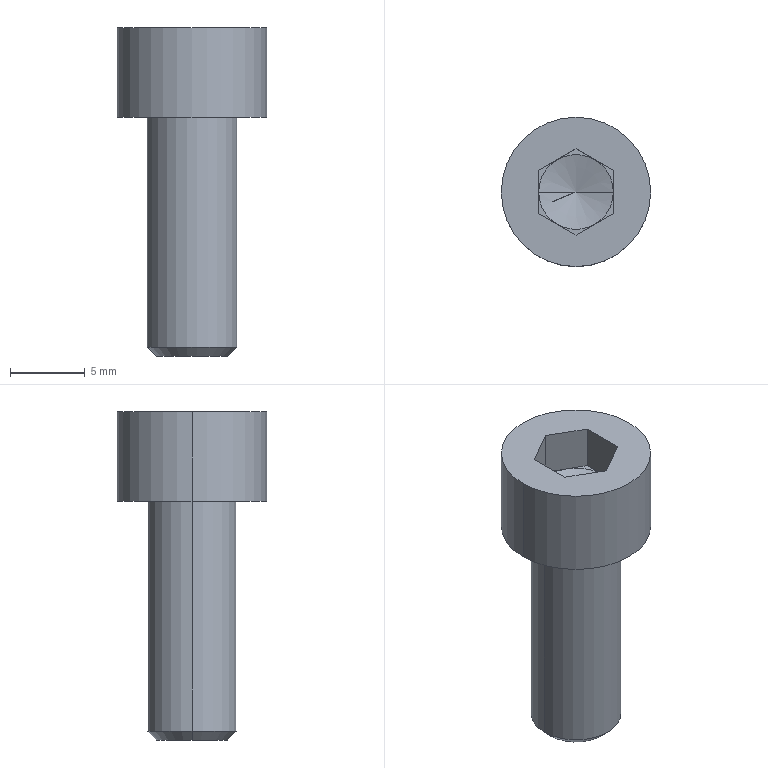Part | STEP file | TNSN20-Y20-F22-Part-7 | 1 solid | 23 faces | box 10 x 10 x 22 mm | volume 850.987 mm3 | plane 15 | cylinder 4 | cone 4 | commonest cylinder face diameters 6 x2 10 x2
STEP:
#1=CARTESIAN_POINT('',(14087.745,13740.046,22.6));
#2=VERTEX_POINT('',#1);
#3=CARTESIAN_POINT('',(14097.745,13740.046,22.6));
#4=VERTEX_POINT('',#3);
#5=CARTESIAN_POINT('',(14092.745,13740.046,22.6));
#6=DIRECTION('',(0.,0.,-1.));
#7=DIRECTION('',(1.,0.,0.));
#8=AXIS2_PLACEMENT_3D('',#5,#6,#7);
#9=CIRCLE('',#8,5.);
#10=EDGE_CURVE('',#2,#4,#9,.T.);
#11=ORIENTED_EDGE('',*,*,#10,.F.);
#12=CARTESIAN_POINT('',(14092.745,13740.046,22.6));
#13=DIRECTION('',(0.,0.,-1.));
#14=DIRECTION('',(1.,0.,0.));
#15=AXIS2_PLACEMENT_3D('',#12,#13,#14);
#16=CIRCLE('',#15,5.);
#17=EDGE_CURVE('',#4,#2,#16,.T.);
#18=ORIENTED_EDGE('',*,*,#17,.F.);
#19=EDGE_LOOP('',(#11,#18));
#20=FACE_OUTER_BOUND('',#19,.T.);
#21=CARTESIAN_POINT('',(14092.745,13742.933,22.6));
#22=VERTEX_POINT('',#21);
#23=CARTESIAN_POINT('',(14095.245,13741.49,22.6));
#24=VERTEX_POINT('',#23);
#25=CARTESIAN_POINT('',(14092.745,13742.933,22.6));
#26=DIRECTION('',(0.866,-0.5,0.));
#27=VECTOR('',#26,1000.);
#28=LINE('',#25,#27);
#29=EDGE_CURVE('',#22,#24,#28,.T.);
#30=ORIENTED_EDGE('',*,*,#29,.T.);
#31=CARTESIAN_POINT('',(14095.245,13738.603,22.6));
#32=VERTEX_POINT('',#31);
#33=CARTESIAN_POINT('',(14095.245,13741.49,22.6));
#34=DIRECTION('',(0.,-1.,0.));
#35=VECTOR('',#34,1000.);
#36=LINE('',#33,#35);
#37=EDGE_CURVE('',#24,#32,#36,.T.);
#38=ORIENTED_EDGE('',*,*,#37,.T.);
#39=CARTESIAN_POINT('',(14092.745,13737.16,22.6));
#40=VERTEX_POINT('',#39);
#41=CARTESIAN_POINT('',(14095.245,13738.603,22.6));
#42=DIRECTION('',(-0.866,-0.5,0.));
#43=VECTOR('',#42,1000.);
#44=LINE('',#41,#43);
#45=EDGE_CURVE('',#32,#40,#44,.T.);
#46=ORIENTED_EDGE('',*,*,#45,.T.);
#47=CARTESIAN_POINT('',(14090.245,13738.603,22.6));
#48=VERTEX_POINT('',#47);
#49=CARTESIAN_POINT('',(14092.745,13737.16,22.6));
#50=DIRECTION('',(-0.866,0.5,0.));
#51=VECTOR('',#50,1000.);
#52=LINE('',#49,#51);
#53=EDGE_CURVE('',#40,#48,#52,.T.);
#54=ORIENTED_EDGE('',*,*,#53,.T.);
#55=CARTESIAN_POINT('',(14090.245,13741.49,22.6));
#56=VERTEX_POINT('',#55);
#57=CARTESIAN_POINT('',(14090.245,13738.603,22.6));
#58=DIRECTION('',(0.,1.,0.));
#59=VECTOR('',#58,1000.);
#60=LINE('',#57,#59);
#61=EDGE_CURVE('',#48,#56,#60,.T.);
#62=ORIENTED_EDGE('',*,*,#61,.T.);
#63=CARTESIAN_POINT('',(14090.245,13741.49,22.6));
#64=DIRECTION('',(0.866,0.5,0.));
#65=VECTOR('',#64,1000.);
#66=LINE('',#63,#65);
#67=EDGE_CURVE('',#56,#22,#66,.T.);
#68=ORIENTED_EDGE('',*,*,#67,.T.);
#69=EDGE_LOOP('',(#30,#38,#46,#54,#62,#68));
#70=FACE_BOUND('',#69,.T.);
#71=CARTESIAN_POINT('',(14073.06,13757.231,22.6));
#72=DIRECTION('',(0.,0.,-1.));
#73=DIRECTION('',(1.,0.,0.));
#74=AXIS2_PLACEMENT_3D('',#71,#72,#73);
#75=PLANE('',#74);
#76=ADVANCED_FACE('',(#20,#70),#75,.F.);
#77=CARTESIAN_POINT('',(14097.745,13740.046,16.6));
#78=VERTEX_POINT('',#77);
#79=CARTESIAN_POINT('',(14087.745,13740.046,16.6));
#80=VERTEX_POINT('',#79);
#81=CARTESIAN_POINT('',(14092.745,13740.046,16.6));
#82=DIRECTION('',(0.,0.,-1.));
#83=DIRECTION('',(1.,0.,0.));
#84=AXIS2_PLACEMENT_3D('',#81,#82,#83);
#85=CIRCLE('',#84,5.);
#86=EDGE_CURVE('',#78,#80,#85,.T.);
#87=ORIENTED_EDGE('',*,*,#86,.T.);
#88=CARTESIAN_POINT('',(14092.745,13740.046,16.6));
#89=DIRECTION('',(0.,0.,-1.));
#90=DIRECTION('',(1.,0.,0.));
#91=AXIS2_PLACEMENT_3D('',#88,#89,#90);
#92=CIRCLE('',#91,5.);
#93=EDGE_CURVE('',#80,#78,#92,.T.);
#94=ORIENTED_EDGE('',*,*,#93,.T.);
#95=EDGE_LOOP('',(#87,#94));
#96=FACE_OUTER_BOUND('',#95,.T.);
#97=CARTESIAN_POINT('',(14089.745,13740.046,16.6));
#98=VERTEX_POINT('',#97);
#99=CARTESIAN_POINT('',(14095.745,13740.046,16.6));
#100=VERTEX_POINT('',#99);
#101=CARTESIAN_POINT('',(14092.745,13740.046,16.6));
#102=DIRECTION('',(0.,0.,-1.));
#103=DIRECTION('',(1.,0.,0.));
#104=AXIS2_PLACEMENT_3D('',#101,#102,#103);
#105=CIRCLE('',#104,3.);
#106=EDGE_CURVE('',#98,#100,#105,.T.);
#107=ORIENTED_EDGE('',*,*,#106,.F.);
#108=CARTESIAN_POINT('',(14092.745,13740.046,16.6));
#109=DIRECTION('',(0.,0.,-1.));
#110=DIRECTION('',(1.,0.,0.));
#111=AXIS2_PLACEMENT_3D('',#108,#109,#110);
#112=CIRCLE('',#111,3.);
#113=EDGE_CURVE('',#100,#98,#112,.T.);
#114=ORIENTED_EDGE('',*,*,#113,.F.);
#115=EDGE_LOOP('',(#107,#114));
#116=FACE_BOUND('',#115,.T.);
#117=CARTESIAN_POINT('',(14107.43,13757.231,16.6));
#118=DIRECTION('',(0.,0.,1.));
#119=DIRECTION('',(-1.,0.,0.));
#120=AXIS2_PLACEMENT_3D('',#117,#118,#119);
#121=PLANE('',#120);
#122=ADVANCED_FACE('',(#96,#116),#121,.F.);
#123=CARTESIAN_POINT('',(14095.131,13740.046,0.6));
#124=VERTEX_POINT('',#123);
#125=CARTESIAN_POINT('',(14090.358,13740.046,0.6));
#126=VERTEX_POINT('',#125);
#127=CARTESIAN_POINT('',(14092.745,13740.046,0.6));
#128=DIRECTION('',(0.,0.,-1.));
#129=DIRECTION('',(1.,0.,0.));
#130=AXIS2_PLACEMENT_3D('',#127,#128,#129);
#131=CIRCLE('',#130,2.387);
#132=EDGE_CURVE('',#124,#126,#131,.T.);
#133=ORIENTED_EDGE('',*,*,#132,.T.);
#134=CARTESIAN_POINT('',(14092.745,13740.046,0.6));
#135=DIRECTION('',(0.,0.,-1.));
#136=DIRECTION('',(1.,0.,0.));
#137=AXIS2_PLACEMENT_3D('',#134,#135,#136);
#138=CIRCLE('',#137,2.387);
#139=EDGE_CURVE('',#126,#124,#138,.T.);
#140=ORIENTED_EDGE('',*,*,#139,.T.);
#141=EDGE_LOOP('',(#133,#140));
#142=FACE_OUTER_BOUND('',#141,.T.);
#143=CARTESIAN_POINT('',(14099.754,13748.249,0.6));
#144=DIRECTION('',(0.,0.,1.));
#145=DIRECTION('',(-1.,0.,0.));
#146=AXIS2_PLACEMENT_3D('',#143,#144,#145);
#147=PLANE('',#146);
#148=ADVANCED_FACE('',(#142),#147,.F.);
#149=ORIENTED_EDGE('',*,*,#61,.F.);
#150=CARTESIAN_POINT('',(14090.245,13738.603,19.6));
#151=VERTEX_POINT('',#150);
#152=CARTESIAN_POINT('',(14090.245,13738.603,19.6));
#153=DIRECTION('',(0.,0.,1.));
#154=VECTOR('',#153,1000.);
#155=LINE('',#152,#154);
#156=EDGE_CURVE('',#151,#48,#155,.T.);
#157=ORIENTED_EDGE('',*,*,#156,.F.);
#158=CARTESIAN_POINT('',(14090.245,13740.046,19.6));
#159=VERTEX_POINT('',#158);
#160=CARTESIAN_POINT('',(14090.245,13738.603,19.6));
#161=DIRECTION('',(0.,1.,0.));
#162=VECTOR('',#161,1000.);
#163=LINE('',#160,#162);
#164=EDGE_CURVE('',#151,#159,#163,.T.);
#165=ORIENTED_EDGE('',*,*,#164,.T.);
#166=CARTESIAN_POINT('',(14090.245,13741.49,19.6));
#167=VERTEX_POINT('',#166);
#168=CARTESIAN_POINT('',(14090.245,13740.046,19.6));
#169=DIRECTION('',(0.,1.,0.));
#170=VECTOR('',#169,1000.);
#171=LINE('',#168,#170);
#172=EDGE_CURVE('',#159,#167,#171,.T.);
#173=ORIENTED_EDGE('',*,*,#172,.T.);
#174=CARTESIAN_POINT('',(14090.245,13741.49,19.6));
#175=DIRECTION('',(0.,0.,1.));
#176=VECTOR('',#175,1000.);
#177=LINE('',#174,#176);
#178=EDGE_CURVE('',#167,#56,#177,.T.);
#179=ORIENTED_EDGE('',*,*,#178,.T.);
#180=EDGE_LOOP('',(#149,#157,#165,#173,#179));
#181=FACE_OUTER_BOUND('',#180,.T.);
#182=CARTESIAN_POINT('',(14090.245,13743.169,17.978));
#183=DIRECTION('',(1.,0.,0.));
#184=DIRECTION('',(0.,0.,1.));
#185=AXIS2_PLACEMENT_3D('',#182,#183,#184);
#186=PLANE('',#185);
#187=ADVANCED_FACE('',(#181),#186,.T.);
#188=ORIENTED_EDGE('',*,*,#67,.F.);
#189=ORIENTED_EDGE('',*,*,#178,.F.);
#190=CARTESIAN_POINT('',(14091.495,13742.211,19.6));
#191=VERTEX_POINT('',#190);
#192=CARTESIAN_POINT('',(14090.245,13741.49,19.6));
#193=DIRECTION('',(0.866,0.5,0.));
#194=VECTOR('',#193,1000.);
#195=LINE('',#192,#194);
#196=EDGE_CURVE('',#167,#191,#195,.T.);
#197=ORIENTED_EDGE('',*,*,#196,.T.);
#198=CARTESIAN_POINT('',(14092.745,13742.933,19.6));
#199=VERTEX_POINT('',#198);
#200=CARTESIAN_POINT('',(14091.495,13742.211,19.6));
#201=DIRECTION('',(0.866,0.5,0.));
#202=VECTOR('',#201,1000.);
#203=LINE('',#200,#202);
#204=EDGE_CURVE('',#191,#199,#203,.T.);
#205=ORIENTED_EDGE('',*,*,#204,.T.);
#206=CARTESIAN_POINT('',(14092.745,13742.933,19.6));
#207=DIRECTION('',(0.,0.,1.));
#208=VECTOR('',#207,1000.);
#209=LINE('',#206,#208);
#210=EDGE_CURVE('',#199,#22,#209,.T.);
#211=ORIENTED_EDGE('',*,*,#210,.T.);
#212=EDGE_LOOP('',(#188,#189,#197,#205,#211));
#213=FACE_OUTER_BOUND('',#212,.T.);
#214=CARTESIAN_POINT('',(14094.199,13743.773,24.222));
#215=DIRECTION('',(0.5,-0.866,0.));
#216=DIRECTION('',(-0.866,-0.5,0.));
#217=AXIS2_PLACEMENT_3D('',#214,#215,#216);
#218=PLANE('',#217);
#219=ADVANCED_FACE('',(#213),#218,.T.);
#220=ORIENTED_EDGE('',*,*,#29,.F.);
#221=ORIENTED_EDGE('',*,*,#210,.F.);
#222=CARTESIAN_POINT('',(14093.995,13742.211,19.6));
#223=VERTEX_POINT('',#222);
#224=CARTESIAN_POINT('',(14092.745,13742.933,19.6));
#225=DIRECTION('',(0.866,-0.5,0.));
#226=VECTOR('',#225,1000.);
#227=LINE('',#224,#226);
#228=EDGE_CURVE('',#199,#223,#227,.T.);
#229=ORIENTED_EDGE('',*,*,#228,.T.);
#230=CARTESIAN_POINT('',(14095.245,13741.49,19.6));
#231=VERTEX_POINT('',#230);
#232=CARTESIAN_POINT('',(14093.995,13742.211,19.6));
#233=DIRECTION('',(0.866,-0.5,0.));
#234=VECTOR('',#233,1000.);
#235=LINE('',#232,#234);
#236=EDGE_CURVE('',#223,#231,#235,.T.);
#237=ORIENTED_EDGE('',*,*,#236,.T.);
#238=CARTESIAN_POINT('',(14095.245,13741.49,19.6));
#239=DIRECTION('',(0.,0.,1.));
#240=VECTOR('',#239,1000.);
#241=LINE('',#238,#240);
#242=EDGE_CURVE('',#231,#24,#241,.T.);
#243=ORIENTED_EDGE('',*,*,#242,.T.);
#244=EDGE_LOOP('',(#220,#221,#229,#237,#243));
#245=FACE_OUTER_BOUND('',#244,.T.);
#246=CARTESIAN_POINT('',(14096.699,13740.65,24.222));
#247=DIRECTION('',(-0.5,-0.866,0.));
#248=DIRECTION('',(-0.866,0.5,0.));
#249=AXIS2_PLACEMENT_3D('',#246,#247,#248);
#250=PLANE('',#249);
#251=ADVANCED_FACE('',(#245),#250,.T.);
#252=ORIENTED_EDGE('',*,*,#37,.F.);
#253=ORIENTED_EDGE('',*,*,#242,.F.);
#254=CARTESIAN_POINT('',(14095.245,13740.046,19.6));
#255=VERTEX_POINT('',#254);
#256=CARTESIAN_POINT('',(14095.245,13741.49,19.6));
#257=DIRECTION('',(0.,-1.,0.));
#258=VECTOR('',#257,1000.);
#259=LINE('',#256,#258);
#260=EDGE_CURVE('',#231,#255,#259,.T.);
#261=ORIENTED_EDGE('',*,*,#260,.T.);
#262=CARTESIAN_POINT('',(14095.245,13738.603,19.6));
#263=VERTEX_POINT('',#262);
#264=CARTESIAN_POINT('',(14095.245,13740.046,19.6));
#265=DIRECTION('',(0.,-1.,0.));
#266=VECTOR('',#265,1000.);
#267=LINE('',#264,#266);
#268=EDGE_CURVE('',#255,#263,#267,.T.);
#269=ORIENTED_EDGE('',*,*,#268,.T.);
#270=CARTESIAN_POINT('',(14095.245,13738.603,19.6));
#271=DIRECTION('',(0.,0.,1.));
#272=VECTOR('',#271,1000.);
#273=LINE('',#270,#272);
#274=EDGE_CURVE('',#263,#32,#273,.T.);
#275=ORIENTED_EDGE('',*,*,#274,.T.);
#276=EDGE_LOOP('',(#252,#253,#261,#269,#275));
#277=FACE_OUTER_BOUND('',#276,.T.);
#278=CARTESIAN_POINT('',(14095.245,13743.169,24.222));
#279=DIRECTION('',(-1.,0.,0.));
#280=DIRECTION('',(0.,0.,-1.));
#281=AXIS2_PLACEMENT_3D('',#278,#279,#280);
#282=PLANE('',#281);
#283=ADVANCED_FACE('',(#277),#282,.T.);
#284=ORIENTED_EDGE('',*,*,#45,.F.);
#285=ORIENTED_EDGE('',*,*,#274,.F.);
#286=CARTESIAN_POINT('',(14093.995,13737.881,19.6));
#287=VERTEX_POINT('',#286);
#288=CARTESIAN_POINT('',(14095.245,13738.603,19.6));
#289=DIRECTION('',(-0.866,-0.5,0.));
#290=VECTOR('',#289,1000.);
#291=LINE('',#288,#290);
#292=EDGE_CURVE('',#263,#287,#291,.T.);
#293=ORIENTED_EDGE('',*,*,#292,.T.);
#294=CARTESIAN_POINT('',(14092.745,13737.16,19.6));
#295=VERTEX_POINT('',#294);
#296=CARTESIAN_POINT('',(14093.995,13737.881,19.6));
#297=DIRECTION('',(-0.866,-0.5,0.));
#298=VECTOR('',#297,1000.);
#299=LINE('',#296,#298);
#300=EDGE_CURVE('',#287,#295,#299,.T.);
#301=ORIENTED_EDGE('',*,*,#300,.T.);
#302=CARTESIAN_POINT('',(14092.745,13737.16,19.6));
#303=DIRECTION('',(0.,0.,1.));
#304=VECTOR('',#303,1000.);
#305=LINE('',#302,#304);
#306=EDGE_CURVE('',#295,#40,#305,.T.);
#307=ORIENTED_EDGE('',*,*,#306,.T.);
#308=EDGE_LOOP('',(#284,#285,#293,#301,#307));
#309=FACE_OUTER_BOUND('',#308,.T.);
#310=CARTESIAN_POINT('',(14091.291,13736.32,24.222));
#311=DIRECTION('',(-0.5,0.866,0.));
#312=DIRECTION('',(0.866,0.5,0.));
#313=AXIS2_PLACEMENT_3D('',#310,#311,#312);
#314=PLANE('',#313);
#315=ADVANCED_FACE('',(#309),#314,.T.);
#316=ORIENTED_EDGE('',*,*,#53,.F.);
#317=ORIENTED_EDGE('',*,*,#306,.F.);
#318=CARTESIAN_POINT('',(14091.495,13737.881,19.6));
#319=VERTEX_POINT('',#318);
#320=CARTESIAN_POINT('',(14092.745,13737.16,19.6));
#321=DIRECTION('',(-0.866,0.5,0.));
#322=VECTOR('',#321,1000.);
#323=LINE('',#320,#322);
#324=EDGE_CURVE('',#295,#319,#323,.T.);
#325=ORIENTED_EDGE('',*,*,#324,.T.);
#326=CARTESIAN_POINT('',(14091.495,13737.881,19.6));
#327=DIRECTION('',(-0.866,0.5,0.));
#328=VECTOR('',#327,1000.);
#329=LINE('',#326,#328);
#330=EDGE_CURVE('',#319,#151,#329,.T.);
#331=ORIENTED_EDGE('',*,*,#330,.T.);
#332=ORIENTED_EDGE('',*,*,#156,.T.);
#333=EDGE_LOOP('',(#316,#317,#325,#331,#332));
#334=FACE_OUTER_BOUND('',#333,.T.);
#335=CARTESIAN_POINT('',(14088.791,13739.443,24.222));
#336=DIRECTION('',(0.5,0.866,0.));
#337=DIRECTION('',(0.866,-0.5,0.));
#338=AXIS2_PLACEMENT_3D('',#335,#336,#337);
#339=PLANE('',#338);
#340=ADVANCED_FACE('',(#334),#339,.T.);
#341=CARTESIAN_POINT('',(14092.745,13740.046,19.6));
#342=DIRECTION('',(0.,0.,-1.));
#343=DIRECTION('',(1.,0.,0.));
#344=AXIS2_PLACEMENT_3D('',#341,#342,#343);
#345=CIRCLE('',#344,2.5);
#346=EDGE_CURVE('',#255,#287,#345,.T.);
#347=ORIENTED_EDGE('',*,*,#346,.T.);
#348=ORIENTED_EDGE('',*,*,#292,.F.);
#349=ORIENTED_EDGE('',*,*,#268,.F.);
#350=EDGE_LOOP('',(#347,#348,#349));
#351=FACE_OUTER_BOUND('',#350,.T.);
#352=CARTESIAN_POINT('',(14092.745,13740.839,19.6));
#353=DIRECTION('',(0.,0.,-1.));
#354=DIRECTION('',(1.,0.,0.));
#355=AXIS2_PLACEMENT_3D('',#352,#353,#354);
#356=PLANE('',#355);
#357=ADVANCED_FACE('',(#351),#356,.F.);
#358=ORIENTED_EDGE('',*,*,#300,.F.);
#359=CARTESIAN_POINT('',(14092.745,13740.046,19.6));
#360=DIRECTION('',(0.,0.,-1.));
#361=DIRECTION('',(0.5,-0.866,0.));
#362=AXIS2_PLACEMENT_3D('',#359,#360,#361);
#363=CIRCLE('',#362,2.5);
#364=EDGE_CURVE('',#287,#319,#363,.T.);
#365=ORIENTED_EDGE('',*,*,#364,.T.);
#366=ORIENTED_EDGE('',*,*,#324,.F.);
#367=EDGE_LOOP('',(#358,#365,#366));
#368=FACE_OUTER_BOUND('',#367,.T.);
#369=CARTESIAN_POINT('',(14090.793,13739.472,19.6));
#370=DIRECTION('',(0.,0.,-1.));
#371=DIRECTION('',(1.,0.,0.));
#372=AXIS2_PLACEMENT_3D('',#369,#370,#371);
#373=PLANE('',#372);
#374=ADVANCED_FACE('',(#368),#373,.F.);
#375=CARTESIAN_POINT('',(14092.745,13740.046,19.6));
#376=DIRECTION('',(0.,0.,-1.));
#377=DIRECTION('',(-0.5,-0.866,0.));
#378=AXIS2_PLACEMENT_3D('',#375,#376,#377);
#379=CIRCLE('',#378,2.5);
#380=EDGE_CURVE('',#319,#159,#379,.T.);
#381=ORIENTED_EDGE('',*,*,#380,.T.);
#382=ORIENTED_EDGE('',*,*,#164,.F.);
#383=ORIENTED_EDGE('',*,*,#330,.F.);
#384=EDGE_LOOP('',(#381,#382,#383));
#385=FACE_OUTER_BOUND('',#384,.T.);
#386=CARTESIAN_POINT('',(14088.995,13740.839,19.6));
#387=DIRECTION('',(0.,0.,-1.));
#388=DIRECTION('',(1.,0.,0.));
#389=AXIS2_PLACEMENT_3D('',#386,#387,#388);
#390=PLANE('',#389);
#391=ADVANCED_FACE('',(#385),#390,.F.);
#392=CARTESIAN_POINT('',(14092.745,13740.046,19.6));
#393=DIRECTION('',(0.,0.,-1.));
#394=DIRECTION('',(-1.,0.,0.));
#395=AXIS2_PLACEMENT_3D('',#392,#393,#394);
#396=CIRCLE('',#395,2.5);
#397=EDGE_CURVE('',#159,#191,#396,.T.);
#398=ORIENTED_EDGE('',*,*,#397,.T.);
#399=ORIENTED_EDGE('',*,*,#196,.F.);
#400=ORIENTED_EDGE('',*,*,#172,.F.);
#401=EDGE_LOOP('',(#398,#399,#400));
#402=FACE_OUTER_BOUND('',#401,.T.);
#403=CARTESIAN_POINT('',(14088.995,13743.004,19.6));
#404=DIRECTION('',(0.,0.,-1.));
#405=DIRECTION('',(1.,0.,0.));
#406=AXIS2_PLACEMENT_3D('',#403,#404,#405);
#407=PLANE('',#406);
#408=ADVANCED_FACE('',(#402),#407,.F.);
#409=CARTESIAN_POINT('',(14092.745,13740.046,19.6));
#410=DIRECTION('',(0.,0.,-1.));
#411=DIRECTION('',(-0.5,0.866,0.));
#412=AXIS2_PLACEMENT_3D('',#409,#410,#411);
#413=CIRCLE('',#412,2.5);
#414=EDGE_CURVE('',#191,#223,#413,.T.);
#415=ORIENTED_EDGE('',*,*,#414,.T.);
#416=ORIENTED_EDGE('',*,*,#228,.F.);
#417=ORIENTED_EDGE('',*,*,#204,.F.);
#418=EDGE_LOOP('',(#415,#416,#417));
#419=FACE_OUTER_BOUND('',#418,.T.);
#420=CARTESIAN_POINT('',(14090.793,13744.524,19.6));
#421=DIRECTION('',(0.,0.,-1.));
#422=DIRECTION('',(1.,0.,0.));
#423=AXIS2_PLACEMENT_3D('',#420,#421,#422);
#424=PLANE('',#423);
#425=ADVANCED_FACE('',(#419),#424,.F.);
#426=CARTESIAN_POINT('',(14092.745,13740.046,19.6));
#427=DIRECTION('',(0.,0.,-1.));
#428=DIRECTION('',(0.5,0.866,0.));
#429=AXIS2_PLACEMENT_3D('',#426,#427,#428);
#430=CIRCLE('',#429,2.5);
#431=EDGE_CURVE('',#223,#255,#430,.T.);
#432=ORIENTED_EDGE('',*,*,#431,.T.);
#433=ORIENTED_EDGE('',*,*,#260,.F.);
#434=ORIENTED_EDGE('',*,*,#236,.F.);
#435=EDGE_LOOP('',(#432,#433,#434));
#436=FACE_OUTER_BOUND('',#435,.T.);
#437=CARTESIAN_POINT('',(14092.745,13743.004,19.6));
#438=DIRECTION('',(0.,0.,-1.));
#439=DIRECTION('',(1.,0.,0.));
#440=AXIS2_PLACEMENT_3D('',#437,#438,#439);
#441=PLANE('',#440);
#442=ADVANCED_FACE('',(#436),#441,.F.);
#443=ORIENTED_EDGE('',*,*,#93,.F.);
#444=CARTESIAN_POINT('',(14087.745,13740.046,22.6));
#445=DIRECTION('',(0.,0.,-1.));
#446=VECTOR('',#445,1000.);
#447=LINE('',#444,#446);
#448=EDGE_CURVE('',#2,#80,#447,.T.);
#449=ORIENTED_EDGE('',*,*,#448,.F.);
#450=ORIENTED_EDGE('',*,*,#10,.T.);
#451=CARTESIAN_POINT('',(14097.745,13740.046,22.6));
#452=DIRECTION('',(0.,0.,-1.));
#453=VECTOR('',#452,1000.);
#454=LINE('',#451,#453);
#455=EDGE_CURVE('',#4,#78,#454,.T.);
#456=ORIENTED_EDGE('',*,*,#455,.T.);
#457=EDGE_LOOP('',(#443,#449,#450,#456));
#458=FACE_OUTER_BOUND('',#457,.T.);
#459=CARTESIAN_POINT('',(14092.745,13740.046,19.6));
#460=DIRECTION('',(0.,0.,-1.));
#461=DIRECTION('',(-1.,0.,0.));
#462=AXIS2_PLACEMENT_3D('',#459,#460,#461);
#463=CYLINDRICAL_SURFACE('',#462,5.);
#464=ADVANCED_FACE('',(#458),#463,.T.);
#465=ORIENTED_EDGE('',*,*,#17,.T.);
#466=ORIENTED_EDGE('',*,*,#448,.T.);
#467=ORIENTED_EDGE('',*,*,#86,.F.);
#468=ORIENTED_EDGE('',*,*,#455,.F.);
#469=EDGE_LOOP('',(#465,#466,#467,#468));
#470=FACE_OUTER_BOUND('',#469,.T.);
#471=CARTESIAN_POINT('',(14092.745,13740.046,19.6));
#472=DIRECTION('',(0.,0.,-1.));
#473=DIRECTION('',(-1.,0.,0.));
#474=AXIS2_PLACEMENT_3D('',#471,#472,#473);
#475=CYLINDRICAL_SURFACE('',#474,5.);
#476=ADVANCED_FACE('',(#470),#475,.T.);
#477=CARTESIAN_POINT('',(14089.745,13740.046,1.213));
#478=VERTEX_POINT('',#477);
#479=CARTESIAN_POINT('',(14095.745,13740.046,1.213));
#480=VERTEX_POINT('',#479);
#481=CARTESIAN_POINT('',(14092.745,13740.046,1.213));
#482=DIRECTION('',(0.,0.,-1.));
#483=DIRECTION('',(1.,0.,0.));
#484=AXIS2_PLACEMENT_3D('',#481,#482,#483);
#485=CIRCLE('',#484,3.);
#486=EDGE_CURVE('',#478,#480,#485,.T.);
#487=ORIENTED_EDGE('',*,*,#486,.F.);
#488=CARTESIAN_POINT('',(14089.745,13740.046,16.6));
#489=DIRECTION('',(0.,0.,-1.));
#490=VECTOR('',#489,1000.);
#491=LINE('',#488,#490);
#492=EDGE_CURVE('',#98,#478,#491,.T.);
#493=ORIENTED_EDGE('',*,*,#492,.F.);
#494=ORIENTED_EDGE('',*,*,#106,.T.);
#495=CARTESIAN_POINT('',(14095.745,13740.046,16.6));
#496=DIRECTION('',(0.,0.,-1.));
#497=VECTOR('',#496,1000.);
#498=LINE('',#495,#497);
#499=EDGE_CURVE('',#100,#480,#498,.T.);
#500=ORIENTED_EDGE('',*,*,#499,.T.);
#501=EDGE_LOOP('',(#487,#493,#494,#500));
#502=FACE_OUTER_BOUND('',#501,.T.);
#503=CARTESIAN_POINT('',(14092.745,13740.046,8.907));
#504=DIRECTION('',(0.,0.,-1.));
#505=DIRECTION('',(-1.,0.,0.));
#506=AXIS2_PLACEMENT_3D('',#503,#504,#505);
#507=CYLINDRICAL_SURFACE('',#506,3.);
#508=ADVANCED_FACE('',(#502),#507,.T.);
#509=ORIENTED_EDGE('',*,*,#113,.T.);
#510=ORIENTED_EDGE('',*,*,#492,.T.);
#511=CARTESIAN_POINT('',(14092.745,13740.046,1.213));
#512=DIRECTION('',(0.,0.,-1.));
#513=DIRECTION('',(1.,0.,0.));
#514=AXIS2_PLACEMENT_3D('',#511,#512,#513);
#515=CIRCLE('',#514,3.);
#516=EDGE_CURVE('',#480,#478,#515,.T.);
#517=ORIENTED_EDGE('',*,*,#516,.F.);
#518=ORIENTED_EDGE('',*,*,#499,.F.);
#519=EDGE_LOOP('',(#509,#510,#517,#518));
#520=FACE_OUTER_BOUND('',#519,.T.);
#521=CARTESIAN_POINT('',(14092.745,13740.046,8.907));
#522=DIRECTION('',(0.,0.,-1.));
#523=DIRECTION('',(-1.,0.,0.));
#524=AXIS2_PLACEMENT_3D('',#521,#522,#523);
#525=CYLINDRICAL_SURFACE('',#524,3.);
#526=ADVANCED_FACE('',(#520),#525,.T.);
#527=ORIENTED_EDGE('',*,*,#139,.F.);
#528=CARTESIAN_POINT('',(14089.745,13740.046,1.214));
#529=DIRECTION('',(0.7071,0.,-0.7071));
#530=VECTOR('',#529,1000.);
#531=LINE('',#528,#530);
#532=EDGE_CURVE('',#478,#126,#531,.T.);
#533=ORIENTED_EDGE('',*,*,#532,.F.);
#534=ORIENTED_EDGE('',*,*,#486,.T.);
#535=CARTESIAN_POINT('',(14095.745,13740.046,1.213));
#536=DIRECTION('',(-0.7071,0.,-0.7071));
#537=VECTOR('',#536,1000.);
#538=LINE('',#535,#537);
#539=EDGE_CURVE('',#480,#124,#538,.T.);
#540=ORIENTED_EDGE('',*,*,#539,.T.);
#541=EDGE_LOOP('',(#527,#533,#534,#540));
#542=FACE_OUTER_BOUND('',#541,.T.);
#543=CARTESIAN_POINT('',(14092.745,13740.046,998.213));
#544=DIRECTION('',(0.,0.,1.));
#545=DIRECTION('',(-1.,0.,0.));
#546=AXIS2_PLACEMENT_3D('',#543,#544,#545);
#547=CONICAL_SURFACE('',#546,1000.,0.7854);
#548=ADVANCED_FACE('',(#542),#547,.T.);
#549=ORIENTED_EDGE('',*,*,#516,.T.);
#550=ORIENTED_EDGE('',*,*,#532,.T.);
#551=ORIENTED_EDGE('',*,*,#132,.F.);
#552=ORIENTED_EDGE('',*,*,#539,.F.);
#553=EDGE_LOOP('',(#549,#550,#551,#552));
#554=FACE_OUTER_BOUND('',#553,.T.);
#555=CARTESIAN_POINT('',(14092.745,13740.046,998.213));
#556=DIRECTION('',(0.,0.,1.));
#557=DIRECTION('',(-1.,0.,0.));
#558=AXIS2_PLACEMENT_3D('',#555,#556,#557);
#559=CONICAL_SURFACE('',#558,1000.,0.7854);
#560=ADVANCED_FACE('',(#554),#559,.T.);
#561=ORIENTED_EDGE('',*,*,#431,.F.);
#562=ORIENTED_EDGE('',*,*,#414,.F.);
#563=ORIENTED_EDGE('',*,*,#397,.F.);
#564=CARTESIAN_POINT('',(14092.745,13740.046,18.93));
#565=VERTEX_POINT('',#564);
#566=CARTESIAN_POINT('',(14090.245,13740.046,19.6));
#567=DIRECTION('',(0.9659,0.,-0.2588));
#568=VECTOR('',#567,1000.);
#569=LINE('',#566,#568);
#570=EDGE_CURVE('',#159,#565,#569,.T.);
#571=ORIENTED_EDGE('',*,*,#570,.T.);
#572=CARTESIAN_POINT('',(14095.245,13740.046,19.6));
#573=DIRECTION('',(-0.9659,0.,-0.2588));
#574=VECTOR('',#573,1000.);
#575=LINE('',#572,#574);
#576=EDGE_CURVE('',#255,#565,#575,.T.);
#577=ORIENTED_EDGE('',*,*,#576,.F.);
#578=EDGE_LOOP('',(#561,#562,#563,#571,#577));
#579=FACE_OUTER_BOUND('',#578,.T.);
#580=CARTESIAN_POINT('',(14092.745,13740.046,1018.93));
#581=DIRECTION('',(0.,0.,1.));
#582=DIRECTION('',(-1.,0.,0.));
#583=AXIS2_PLACEMENT_3D('',#580,#581,#582);
#584=CONICAL_SURFACE('',#583,3732.051,1.309);
#585=ADVANCED_FACE('',(#579),#584,.F.);
#586=ORIENTED_EDGE('',*,*,#570,.F.);
#587=ORIENTED_EDGE('',*,*,#380,.F.);
#588=ORIENTED_EDGE('',*,*,#364,.F.);
#589=ORIENTED_EDGE('',*,*,#346,.F.);
#590=ORIENTED_EDGE('',*,*,#576,.T.);
#591=EDGE_LOOP('',(#586,#587,#588,#589,#590));
#592=FACE_OUTER_BOUND('',#591,.T.);
#593=CARTESIAN_POINT('',(14092.745,13740.046,1018.93));
#594=DIRECTION('',(0.,0.,1.));
#595=DIRECTION('',(-1.,0.,0.));
#596=AXIS2_PLACEMENT_3D('',#593,#594,#595);
#597=CONICAL_SURFACE('',#596,3732.051,1.309);
#598=ADVANCED_FACE('',(#592),#597,.F.);
#599=CLOSED_SHELL('',(#76,#122,#148,#187,#219,#251,#283,#315,#340,#357,#374,#391,#408,#425,#442,#464,#476,#508,#526,#548,#560,#585,#598));
#600=MANIFOLD_SOLID_BREP('',#599);
#601=CARTESIAN_POINT('',(0.,0.,0.));
#602=DIRECTION('',(0.,0.,1.));
#603=DIRECTION('',(1.,0.,0.));
#604=AXIS2_PLACEMENT_3D('',#601,#602,#603);
#605=(LENGTH_UNIT()NAMED_UNIT(*)SI_UNIT(.MILLI.,.METRE.));
#606=UNCERTAINTY_MEASURE_WITH_UNIT(LENGTH_MEASURE(0.00001),#605,'','');
#607=(NAMED_UNIT(*)PLANE_ANGLE_UNIT()SI_UNIT($,.RADIAN.));
#608=(NAMED_UNIT(*)SI_UNIT($,.STERADIAN.)SOLID_ANGLE_UNIT());
#609=(GEOMETRIC_REPRESENTATION_CONTEXT(3)GLOBAL_UNCERTAINTY_ASSIGNED_CONTEXT((#606))GLOBAL_UNIT_ASSIGNED_CONTEXT((#605,#607,#608))REPRESENTATION_CONTEXT('',''));
#610=ADVANCED_BREP_SHAPE_REPRESENTATION('',(#600,#604),#609);